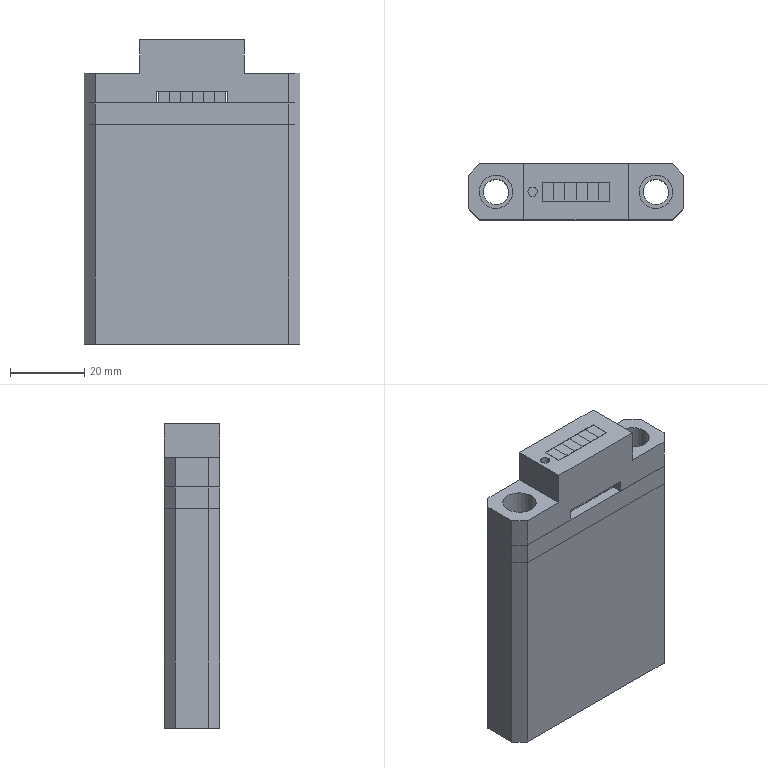Part | CATIA | 9 solids | 116 faces | box 58 x 15 x 81.9 mm | volume 59314 mm3 | plane 102 | cylinder 14 | commonest cylinder face diameters 9 x8 6.8 x4 2.5 x2